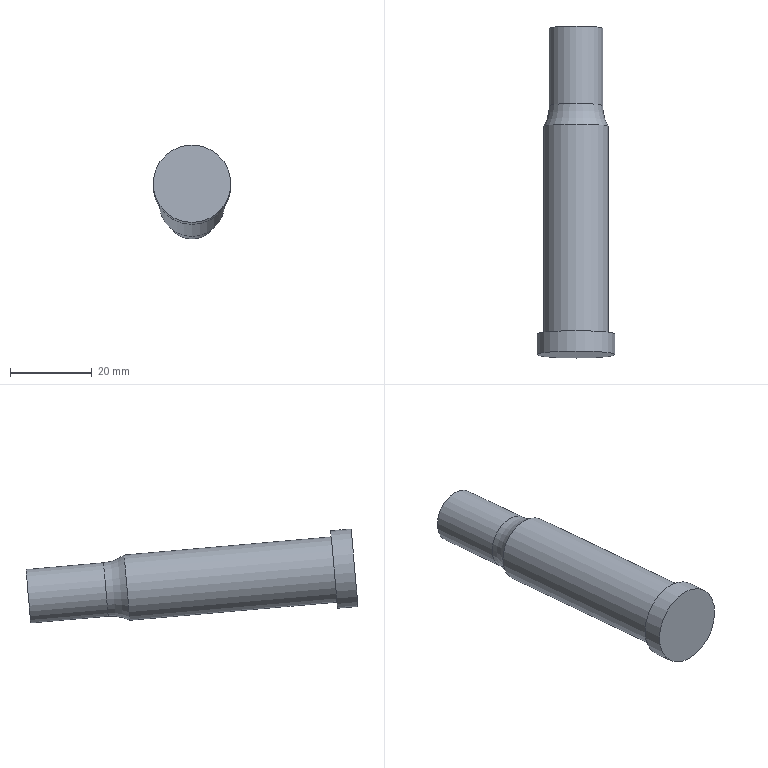Part | NX | features SPAS 16-80-13.10 2 | 1 solid | 7 faces | box 19 x 81.094 x 22.961 mm | volume 15001 mm3 | plane 3 | cylinder 3 | torus 1 | commonest cylinder face diameters 13.1 x1 16 x1 19 x1
STEP:
#1=CARTESIAN_POINT('',(-120.452,-41.84,-43.962));
#2=VERTEX_POINT('',#1);
#3=CARTESIAN_POINT('',(-120.452,-41.27,-37.436));
#4=DIRECTION('',(0.,-0.9962,0.08716));
#5=DIRECTION('',(0.,-0.08716,-0.9962));
#6=AXIS2_PLACEMENT_3D('',#3,#4,#5);
#7=CIRCLE('',#6,6.55);
#8=EDGE_CURVE('',#2,#2,#7,.T.);
#9=ORIENTED_EDGE('',*,*,#8,.F.);
#10=EDGE_LOOP('',(#9));
#11=FACE_BOUND('',#10,.T.);
#12=CARTESIAN_POINT('',(-120.452,-41.27,-37.436));
#13=DIRECTION('',(0.,0.9962,-0.08716));
#14=DIRECTION('',(0.,0.08716,0.9962));
#15=AXIS2_PLACEMENT_3D('',#12,#13,#14);
#16=PLANE('',#15);
#17=ADVANCED_FACE('',(#11),#16,.T.);
#18=CARTESIAN_POINT('',(-120.452,-60.768,-42.306));
#19=VERTEX_POINT('',#18);
#20=CARTESIAN_POINT('',(-120.452,-60.197,-35.781));
#21=DIRECTION('',(0.,-0.9962,0.08716));
#22=DIRECTION('',(0.,-0.08716,-0.9962));
#23=AXIS2_PLACEMENT_3D('',#20,#21,#22);
#24=CIRCLE('',#23,6.55);
#25=EDGE_CURVE('',#19,#19,#24,.F.);
#26=ORIENTED_EDGE('',*,*,#25,.T.);
#27=EDGE_LOOP('',(#26));
#28=FACE_BOUND('',#27,.T.);
#29=ORIENTED_EDGE('',*,*,#8,.T.);
#30=EDGE_LOOP('',(#29));
#31=FACE_BOUND('',#30,.T.);
#32=CARTESIAN_POINT('',(-120.452,-41.27,-37.436));
#33=DIRECTION('',(0.,-0.9962,0.08716));
#34=DIRECTION('',(0.,-0.08716,-0.9962));
#35=AXIS2_PLACEMENT_3D('',#32,#33,#34);
#36=CYLINDRICAL_SURFACE('',#35,6.55);
#37=ADVANCED_FACE('',(#28,#31),#36,.T.);
#38=CARTESIAN_POINT('',(-120.452,-115.287,-22.93));
#39=VERTEX_POINT('',#38);
#40=CARTESIAN_POINT('',(-120.452,-115.984,-30.9));
#41=DIRECTION('',(0.,0.9962,-0.08716));
#42=DIRECTION('',(0.,0.08716,0.9962));
#43=AXIS2_PLACEMENT_3D('',#40,#41,#42);
#44=CIRCLE('',#43,8.);
#45=EDGE_CURVE('',#39,#39,#44,.F.);
#46=ORIENTED_EDGE('',*,*,#45,.F.);
#47=EDGE_LOOP('',(#46));
#48=FACE_BOUND('',#47,.T.);
#49=CARTESIAN_POINT('',(-120.452,-66.061,-43.298));
#50=VERTEX_POINT('',#49);
#51=CARTESIAN_POINT('',(-120.452,-65.364,-35.329));
#52=DIRECTION('',(0.,-0.9962,0.08716));
#53=DIRECTION('',(0.,-0.08716,-0.9962));
#54=AXIS2_PLACEMENT_3D('',#51,#52,#53);
#55=CIRCLE('',#54,8.);
#56=EDGE_CURVE('',#50,#50,#55,.T.);
#57=ORIENTED_EDGE('',*,*,#56,.T.);
#58=EDGE_LOOP('',(#57));
#59=FACE_BOUND('',#58,.T.);
#60=CARTESIAN_POINT('',(-120.452,-65.364,-35.329));
#61=DIRECTION('',(0.,-0.9962,0.08716));
#62=DIRECTION('',(0.,-0.08716,-0.9962));
#63=AXIS2_PLACEMENT_3D('',#60,#61,#62);
#64=CYLINDRICAL_SURFACE('',#63,8.);
#65=ADVANCED_FACE('',(#48,#59),#64,.T.);
#66=CARTESIAN_POINT('',(-120.452,-120.137,-21.));
#67=VERTEX_POINT('',#66);
#68=CARTESIAN_POINT('',(-120.452,-120.965,-30.464));
#69=DIRECTION('',(0.,0.9962,-0.08716));
#70=DIRECTION('',(0.,0.08716,0.9962));
#71=AXIS2_PLACEMENT_3D('',#68,#69,#70);
#72=CIRCLE('',#71,9.5);
#73=EDGE_CURVE('',#67,#67,#72,.T.);
#74=ORIENTED_EDGE('',*,*,#73,.F.);
#75=EDGE_LOOP('',(#74));
#76=FACE_BOUND('',#75,.T.);
#77=CARTESIAN_POINT('',(-120.452,-120.965,-30.464));
#78=DIRECTION('',(0.,-0.9962,0.08716));
#79=DIRECTION('',(0.,-0.08716,-0.9962));
#80=AXIS2_PLACEMENT_3D('',#77,#78,#79);
#81=PLANE('',#80);
#82=ADVANCED_FACE('',(#76),#81,.T.);
#83=ORIENTED_EDGE('',*,*,#45,.T.);
#84=EDGE_LOOP('',(#83));
#85=FACE_BOUND('',#84,.T.);
#86=CARTESIAN_POINT('',(-120.452,-116.812,-40.364));
#87=VERTEX_POINT('',#86);
#88=CARTESIAN_POINT('',(-120.452,-115.984,-30.9));
#89=DIRECTION('',(0.,-0.9962,0.08716));
#90=DIRECTION('',(0.,-0.08716,-0.9962));
#91=AXIS2_PLACEMENT_3D('',#88,#89,#90);
#92=CIRCLE('',#91,9.5);
#93=EDGE_CURVE('',#87,#87,#92,.T.);
#94=ORIENTED_EDGE('',*,*,#93,.F.);
#95=EDGE_LOOP('',(#94));
#96=FACE_BOUND('',#95,.T.);
#97=CARTESIAN_POINT('',(-120.452,-115.984,-30.9));
#98=DIRECTION('',(0.,0.9962,-0.08716));
#99=DIRECTION('',(0.,0.08716,0.9962));
#100=AXIS2_PLACEMENT_3D('',#97,#98,#99);
#101=PLANE('',#100);
#102=ADVANCED_FACE('',(#85,#96),#101,.T.);
#103=ORIENTED_EDGE('',*,*,#73,.T.);
#104=EDGE_LOOP('',(#103));
#105=FACE_BOUND('',#104,.T.);
#106=ORIENTED_EDGE('',*,*,#93,.T.);
#107=EDGE_LOOP('',(#106));
#108=FACE_BOUND('',#107,.T.);
#109=CARTESIAN_POINT('',(-120.452,-115.984,-30.9));
#110=DIRECTION('',(0.,-0.9962,0.08716));
#111=DIRECTION('',(0.,-0.08716,-0.9962));
#112=AXIS2_PLACEMENT_3D('',#109,#110,#111);
#113=CYLINDRICAL_SURFACE('',#112,9.5);
#114=ADVANCED_FACE('',(#105,#108),#113,.T.);
#115=ORIENTED_EDGE('',*,*,#25,.F.);
#116=EDGE_LOOP('',(#115));
#117=FACE_BOUND('',#116,.T.);
#118=ORIENTED_EDGE('',*,*,#56,.F.);
#119=EDGE_LOOP('',(#118));
#120=FACE_BOUND('',#119,.T.);
#121=CARTESIAN_POINT('',(-120.452,-60.197,-35.781));
#122=DIRECTION('',(0.,-0.9962,0.08716));
#123=DIRECTION('',(0.,-0.08716,-0.9962));
#124=AXIS2_PLACEMENT_3D('',#121,#122,#123);
#125=TOROIDAL_SURFACE('',#124,16.55,10.);
#126=ADVANCED_FACE('',(#117,#120),#125,.F.);
#127=CLOSED_SHELL('',(#17,#37,#65,#82,#102,#114,#126));
#128=MANIFOLD_SOLID_BREP('',#127);
#129=(LENGTH_UNIT()NAMED_UNIT(*)SI_UNIT(.MILLI.,.METRE.));
#130=UNCERTAINTY_MEASURE_WITH_UNIT(LENGTH_MEASURE(0.00001),#129,'','');
#131=(NAMED_UNIT(*)PLANE_ANGLE_UNIT()SI_UNIT($,.RADIAN.));
#132=(NAMED_UNIT(*)SI_UNIT($,.STERADIAN.)SOLID_ANGLE_UNIT());
#133=(GEOMETRIC_REPRESENTATION_CONTEXT(3)GLOBAL_UNCERTAINTY_ASSIGNED_CONTEXT((#130))GLOBAL_UNIT_ASSIGNED_CONTEXT((#129,#131,#132))REPRESENTATION_CONTEXT('',''));
#134=ADVANCED_BREP_SHAPE_REPRESENTATION('',(#128),#133);